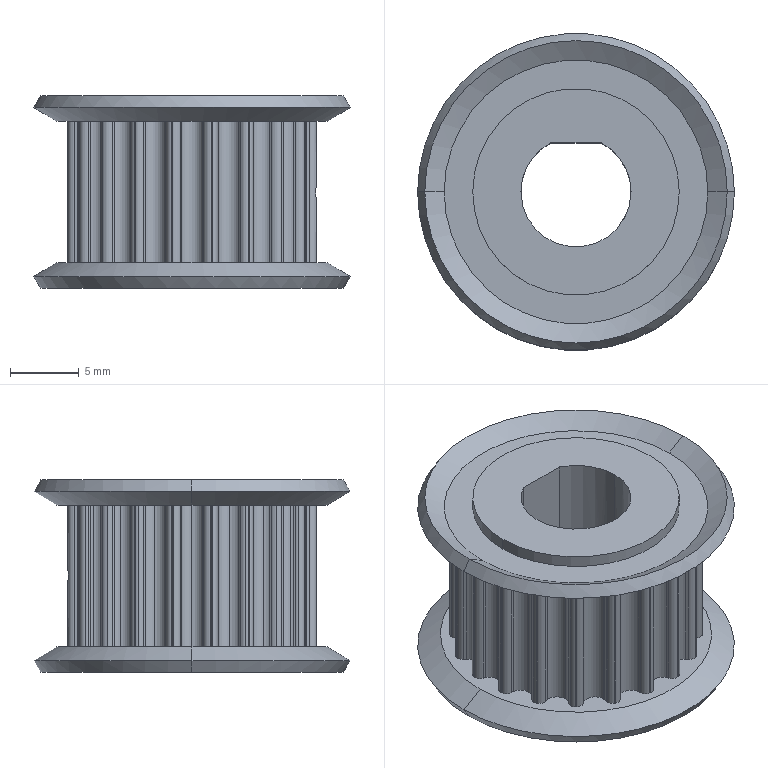Part | NX | features BREP 1 | 1 solid | 184 faces | box 23 x 23 x 14 mm | volume 2723 mm3 | cylinder 165 | cone 12 | plane 7 | commonest cylinder face diameters 1.02 x55 3.04 x46 1.7 x29 18.34 x24 3.3 x4 15 x4